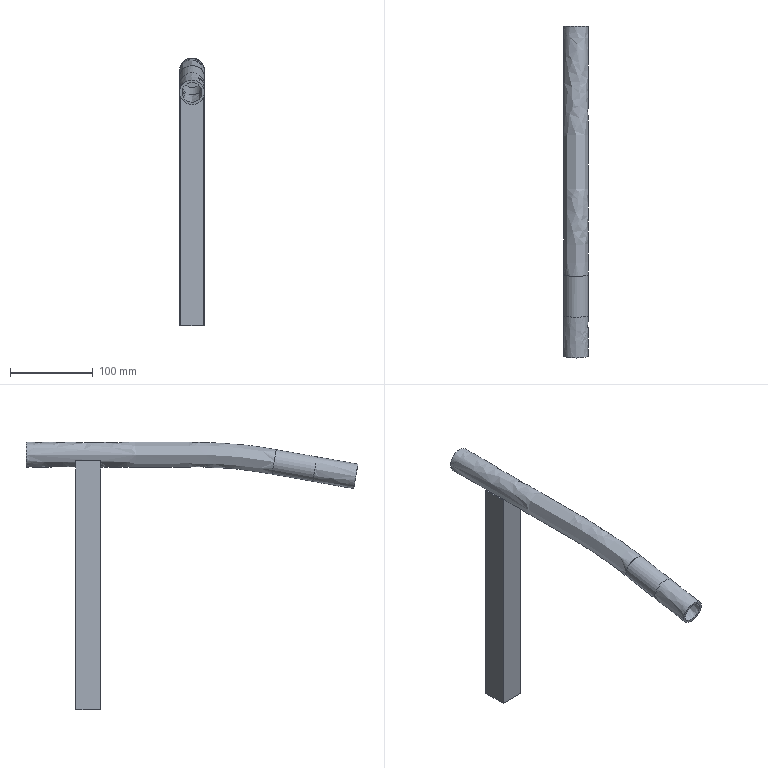Part | NX | features solid 2 | 1 solid | 22 faces | box 30 x 400.326 x 322.586 mm | volume 154131 mm3 | plane 15 | spline 4 | cylinder 3 | commonest cylinder face diameters 30 x2 24 x1
STEP:
#1=CARTESIAN_POINT('',(-652.509,-944.,-115.));
#2=VERTEX_POINT('',#1);
#3=CARTESIAN_POINT('',(-678.491,-944.,-115.));
#4=VERTEX_POINT('',#3);
#5=CARTESIAN_POINT('',(-652.509,-944.,-115.));
#6=CARTESIAN_POINT('',(-653.831,-944.,-117.288));
#7=CARTESIAN_POINT('',(-657.637,-944.,-121.084));
#8=CARTESIAN_POINT('',(-665.504,-944.,-123.205));
#9=CARTESIAN_POINT('',(-673.339,-944.,-121.096));
#10=CARTESIAN_POINT('',(-677.169,-944.,-117.288));
#11=CARTESIAN_POINT('',(-678.491,-944.,-115.));
#12=B_SPLINE_CURVE_WITH_KNOTS('',3,(#5,#6,#7,#8,#9,#10,#11),.UNSPECIFIED.,.F.,.F.,(4,1,1,1,4),(0.,0.007815,0.01563,0.02344,0.03126),.UNSPECIFIED.);
#13=EDGE_CURVE('',#2,#4,#12,.T.);
#14=ORIENTED_EDGE('',*,*,#13,.T.);
#15=CARTESIAN_POINT('',(-680.5,-944.,-115.));
#16=VERTEX_POINT('',#15);
#17=CARTESIAN_POINT('',(-680.5,-944.,-115.));
#18=DIRECTION('',(-1.,0.,0.));
#19=VECTOR('',#18,1000.);
#20=LINE('',#17,#19);
#21=EDGE_CURVE('',#16,#4,#20,.F.);
#22=ORIENTED_EDGE('',*,*,#21,.F.);
#23=CARTESIAN_POINT('',(-680.5,-944.,-415.));
#24=VERTEX_POINT('',#23);
#25=CARTESIAN_POINT('',(-680.5,-944.,-400.));
#26=DIRECTION('',(0.,0.,1.));
#27=VECTOR('',#26,1000.);
#28=LINE('',#25,#27);
#29=EDGE_CURVE('',#24,#16,#28,.T.);
#30=ORIENTED_EDGE('',*,*,#29,.F.);
#31=CARTESIAN_POINT('',(-650.5,-944.,-415.));
#32=VERTEX_POINT('',#31);
#33=CARTESIAN_POINT('',(-683.25,-944.,-415.));
#34=DIRECTION('',(-1.,0.,0.));
#35=VECTOR('',#34,1000.);
#36=LINE('',#33,#35);
#37=EDGE_CURVE('',#24,#32,#36,.F.);
#38=ORIENTED_EDGE('',*,*,#37,.T.);
#39=CARTESIAN_POINT('',(-650.5,-944.,-115.));
#40=VERTEX_POINT('',#39);
#41=CARTESIAN_POINT('',(-650.5,-944.,-400.));
#42=DIRECTION('',(0.,0.,-1.));
#43=VECTOR('',#42,1000.);
#44=LINE('',#41,#43);
#45=EDGE_CURVE('',#32,#40,#44,.F.);
#46=ORIENTED_EDGE('',*,*,#45,.T.);
#47=CARTESIAN_POINT('',(-680.5,-944.,-115.));
#48=DIRECTION('',(-1.,0.,0.));
#49=VECTOR('',#48,1000.);
#50=LINE('',#47,#49);
#51=EDGE_CURVE('',#2,#40,#50,.F.);
#52=ORIENTED_EDGE('',*,*,#51,.F.);
#53=EDGE_LOOP('',(#14,#22,#30,#38,#46,#52));
#54=FACE_BOUND('',#53,.T.);
#55=CARTESIAN_POINT('',(-683.25,-944.,-400.));
#56=DIRECTION('',(0.,1.,0.));
#57=DIRECTION('',(1.,0.,0.));
#58=AXIS2_PLACEMENT_3D('',#55,#56,#57);
#59=PLANE('',#58);
#60=ADVANCED_FACE('',(#54),#59,.F.);
#61=CARTESIAN_POINT('',(-678.49,-942.5,-115.));
#62=VERTEX_POINT('',#61);
#63=CARTESIAN_POINT('',(-652.51,-942.5,-115.));
#64=VERTEX_POINT('',#63);
#65=CARTESIAN_POINT('',(-678.49,-942.5,-115.));
#66=CARTESIAN_POINT('',(-677.169,-942.5,-117.288));
#67=CARTESIAN_POINT('',(-673.363,-942.5,-121.084));
#68=CARTESIAN_POINT('',(-665.496,-942.5,-123.205));
#69=CARTESIAN_POINT('',(-657.661,-942.5,-121.096));
#70=CARTESIAN_POINT('',(-653.831,-942.5,-117.288));
#71=CARTESIAN_POINT('',(-652.51,-942.5,-115.));
#72=B_SPLINE_CURVE_WITH_KNOTS('',3,(#65,#66,#67,#68,#69,#70,#71),.UNSPECIFIED.,.F.,.F.,(4,1,1,1,4),(0.,0.007814,0.01563,0.02344,0.03126),.UNSPECIFIED.);
#73=EDGE_CURVE('',#62,#64,#72,.T.);
#74=ORIENTED_EDGE('',*,*,#73,.T.);
#75=CARTESIAN_POINT('',(-652.,-942.5,-115.));
#76=VERTEX_POINT('',#75);
#77=CARTESIAN_POINT('',(-683.25,-942.5,-115.));
#78=DIRECTION('',(-1.,0.,0.));
#79=VECTOR('',#78,1000.);
#80=LINE('',#77,#79);
#81=EDGE_CURVE('',#76,#64,#80,.T.);
#82=ORIENTED_EDGE('',*,*,#81,.F.);
#83=CARTESIAN_POINT('',(-652.,-942.5,-415.));
#84=VERTEX_POINT('',#83);
#85=CARTESIAN_POINT('',(-652.,-942.5,-50.));
#86=DIRECTION('',(0.,0.,-1.));
#87=VECTOR('',#86,1000.);
#88=LINE('',#85,#87);
#89=EDGE_CURVE('',#76,#84,#88,.T.);
#90=ORIENTED_EDGE('',*,*,#89,.T.);
#91=CARTESIAN_POINT('',(-679.,-942.5,-415.));
#92=VERTEX_POINT('',#91);
#93=CARTESIAN_POINT('',(-683.25,-942.5,-415.));
#94=DIRECTION('',(1.,0.,0.));
#95=VECTOR('',#94,1000.);
#96=LINE('',#93,#95);
#97=EDGE_CURVE('',#84,#92,#96,.F.);
#98=ORIENTED_EDGE('',*,*,#97,.T.);
#99=CARTESIAN_POINT('',(-679.,-942.5,-115.));
#100=VERTEX_POINT('',#99);
#101=CARTESIAN_POINT('',(-679.,-942.5,-50.));
#102=DIRECTION('',(0.,0.,-1.));
#103=VECTOR('',#102,1000.);
#104=LINE('',#101,#103);
#105=EDGE_CURVE('',#100,#92,#104,.T.);
#106=ORIENTED_EDGE('',*,*,#105,.F.);
#107=CARTESIAN_POINT('',(-683.25,-942.5,-115.));
#108=DIRECTION('',(-1.,0.,0.));
#109=VECTOR('',#108,1000.);
#110=LINE('',#107,#109);
#111=EDGE_CURVE('',#62,#100,#110,.T.);
#112=ORIENTED_EDGE('',*,*,#111,.F.);
#113=EDGE_LOOP('',(#74,#82,#90,#98,#106,#112));
#114=FACE_BOUND('',#113,.T.);
#115=CARTESIAN_POINT('',(-683.25,-942.5,-50.));
#116=DIRECTION('',(0.,-1.,0.));
#117=DIRECTION('',(-1.,0.,0.));
#118=AXIS2_PLACEMENT_3D('',#115,#116,#117);
#119=PLANE('',#118);
#120=ADVANCED_FACE('',(#114),#119,.F.);
#121=CARTESIAN_POINT('',(-652.509,-944.,-115.));
#122=CARTESIAN_POINT('',(-652.51,-943.5,-115.));
#123=CARTESIAN_POINT('',(-652.51,-943.,-115.));
#124=CARTESIAN_POINT('',(-652.51,-942.5,-115.));
#125=B_SPLINE_CURVE_WITH_KNOTS('',3,(#121,#122,#123,#124),.UNSPECIFIED.,.F.,.F.,(4,4),(0.,0.0015),.UNSPECIFIED.);
#126=EDGE_CURVE('',#64,#2,#125,.F.);
#127=ORIENTED_EDGE('',*,*,#126,.T.);
#128=ORIENTED_EDGE('',*,*,#51,.T.);
#129=CARTESIAN_POINT('',(-650.5,-914.,-115.));
#130=VERTEX_POINT('',#129);
#131=CARTESIAN_POINT('',(-650.5,-914.,-115.));
#132=DIRECTION('',(0.,-1.,0.));
#133=VECTOR('',#132,1000.);
#134=LINE('',#131,#133);
#135=EDGE_CURVE('',#40,#130,#134,.F.);
#136=ORIENTED_EDGE('',*,*,#135,.T.);
#137=CARTESIAN_POINT('',(-652.51,-914.,-115.));
#138=VERTEX_POINT('',#137);
#139=CARTESIAN_POINT('',(-680.5,-914.,-115.));
#140=DIRECTION('',(-1.,0.,0.));
#141=VECTOR('',#140,1000.);
#142=LINE('',#139,#141);
#143=EDGE_CURVE('',#138,#130,#142,.F.);
#144=ORIENTED_EDGE('',*,*,#143,.F.);
#145=CARTESIAN_POINT('',(-652.51,-915.5,-115.));
#146=VERTEX_POINT('',#145);
#147=CARTESIAN_POINT('',(-652.51,-544.,-115.));
#148=DIRECTION('',(0.,-1.,0.));
#149=VECTOR('',#148,1000.);
#150=LINE('',#147,#149);
#151=EDGE_CURVE('',#138,#146,#150,.T.);
#152=ORIENTED_EDGE('',*,*,#151,.T.);
#153=CARTESIAN_POINT('',(-652.,-915.5,-115.));
#154=VERTEX_POINT('',#153);
#155=CARTESIAN_POINT('',(-683.25,-915.5,-115.));
#156=DIRECTION('',(-1.,0.,0.));
#157=VECTOR('',#156,1000.);
#158=LINE('',#155,#157);
#159=EDGE_CURVE('',#154,#146,#158,.T.);
#160=ORIENTED_EDGE('',*,*,#159,.F.);
#161=CARTESIAN_POINT('',(-652.,-914.,-115.));
#162=DIRECTION('',(0.,1.,0.));
#163=VECTOR('',#162,1000.);
#164=LINE('',#161,#163);
#165=EDGE_CURVE('',#76,#154,#164,.T.);
#166=ORIENTED_EDGE('',*,*,#165,.F.);
#167=ORIENTED_EDGE('',*,*,#81,.T.);
#168=EDGE_LOOP('',(#127,#128,#136,#144,#152,#160,#166,#167));
#169=FACE_BOUND('',#168,.T.);
#170=CARTESIAN_POINT('',(-680.5,-914.,-115.));
#171=DIRECTION('',(0.,0.,-1.));
#172=DIRECTION('',(0.,1.,0.));
#173=AXIS2_PLACEMENT_3D('',#170,#171,#172);
#174=PLANE('',#173);
#175=ADVANCED_FACE('',(#169),#174,.F.);
#176=CARTESIAN_POINT('',(-678.491,-944.,-115.));
#177=CARTESIAN_POINT('',(-678.49,-943.5,-115.));
#178=CARTESIAN_POINT('',(-678.49,-943.,-115.));
#179=CARTESIAN_POINT('',(-678.49,-942.5,-115.));
#180=B_SPLINE_CURVE_WITH_KNOTS('',3,(#176,#177,#178,#179),.UNSPECIFIED.,.F.,.F.,(4,4),(0.,0.0015),.UNSPECIFIED.);
#181=EDGE_CURVE('',#4,#62,#180,.T.);
#182=ORIENTED_EDGE('',*,*,#181,.T.);
#183=ORIENTED_EDGE('',*,*,#111,.T.);
#184=CARTESIAN_POINT('',(-679.,-915.5,-115.));
#185=VERTEX_POINT('',#184);
#186=CARTESIAN_POINT('',(-679.,-914.,-115.));
#187=DIRECTION('',(0.,1.,0.));
#188=VECTOR('',#187,1000.);
#189=LINE('',#186,#188);
#190=EDGE_CURVE('',#100,#185,#189,.T.);
#191=ORIENTED_EDGE('',*,*,#190,.T.);
#192=CARTESIAN_POINT('',(-678.49,-915.5,-115.));
#193=VERTEX_POINT('',#192);
#194=CARTESIAN_POINT('',(-683.25,-915.5,-115.));
#195=DIRECTION('',(-1.,0.,0.));
#196=VECTOR('',#195,1000.);
#197=LINE('',#194,#196);
#198=EDGE_CURVE('',#193,#185,#197,.T.);
#199=ORIENTED_EDGE('',*,*,#198,.F.);
#200=CARTESIAN_POINT('',(-678.49,-914.,-115.));
#201=VERTEX_POINT('',#200);
#202=CARTESIAN_POINT('',(-678.49,-544.,-115.));
#203=DIRECTION('',(0.,-1.,0.));
#204=VECTOR('',#203,1000.);
#205=LINE('',#202,#204);
#206=EDGE_CURVE('',#193,#201,#205,.F.);
#207=ORIENTED_EDGE('',*,*,#206,.T.);
#208=CARTESIAN_POINT('',(-680.5,-914.,-115.));
#209=VERTEX_POINT('',#208);
#210=CARTESIAN_POINT('',(-680.5,-914.,-115.));
#211=DIRECTION('',(-1.,0.,0.));
#212=VECTOR('',#211,1000.);
#213=LINE('',#210,#212);
#214=EDGE_CURVE('',#209,#201,#213,.F.);
#215=ORIENTED_EDGE('',*,*,#214,.F.);
#216=CARTESIAN_POINT('',(-680.5,-914.,-115.));
#217=DIRECTION('',(0.,1.,0.));
#218=VECTOR('',#217,1000.);
#219=LINE('',#216,#218);
#220=EDGE_CURVE('',#209,#16,#219,.F.);
#221=ORIENTED_EDGE('',*,*,#220,.T.);
#222=ORIENTED_EDGE('',*,*,#21,.T.);
#223=EDGE_LOOP('',(#182,#183,#191,#199,#207,#215,#221,#222));
#224=FACE_BOUND('',#223,.T.);
#225=CARTESIAN_POINT('',(-680.5,-914.,-115.));
#226=DIRECTION('',(0.,0.,-1.));
#227=DIRECTION('',(0.,1.,0.));
#228=AXIS2_PLACEMENT_3D('',#225,#226,#227);
#229=PLANE('',#228);
#230=ADVANCED_FACE('',(#224),#229,.F.);
#231=CARTESIAN_POINT('',(-680.5,-914.,-415.));
#232=VERTEX_POINT('',#231);
#233=CARTESIAN_POINT('',(-680.5,-914.,-415.));
#234=DIRECTION('',(0.,1.,0.));
#235=VECTOR('',#234,1000.);
#236=LINE('',#233,#235);
#237=EDGE_CURVE('',#232,#24,#236,.F.);
#238=ORIENTED_EDGE('',*,*,#237,.F.);
#239=CARTESIAN_POINT('',(-650.5,-914.,-415.));
#240=VERTEX_POINT('',#239);
#241=CARTESIAN_POINT('',(-683.25,-914.,-415.));
#242=DIRECTION('',(-1.,0.,0.));
#243=VECTOR('',#242,1000.);
#244=LINE('',#241,#243);
#245=EDGE_CURVE('',#232,#240,#244,.F.);
#246=ORIENTED_EDGE('',*,*,#245,.T.);
#247=CARTESIAN_POINT('',(-650.5,-914.,-415.));
#248=DIRECTION('',(0.,-1.,0.));
#249=VECTOR('',#248,1000.);
#250=LINE('',#247,#249);
#251=EDGE_CURVE('',#240,#32,#250,.T.);
#252=ORIENTED_EDGE('',*,*,#251,.T.);
#253=ORIENTED_EDGE('',*,*,#37,.F.);
#254=EDGE_LOOP('',(#238,#246,#252,#253));
#255=FACE_BOUND('',#254,.T.);
#256=CARTESIAN_POINT('',(-652.,-915.5,-415.));
#257=VERTEX_POINT('',#256);
#258=CARTESIAN_POINT('',(-652.,-914.,-415.));
#259=DIRECTION('',(0.,-1.,0.));
#260=VECTOR('',#259,1000.);
#261=LINE('',#258,#260);
#262=EDGE_CURVE('',#84,#257,#261,.F.);
#263=ORIENTED_EDGE('',*,*,#262,.T.);
#264=CARTESIAN_POINT('',(-679.,-915.5,-415.));
#265=VERTEX_POINT('',#264);
#266=CARTESIAN_POINT('',(-683.25,-915.5,-415.));
#267=DIRECTION('',(1.,0.,0.));
#268=VECTOR('',#267,1000.);
#269=LINE('',#266,#268);
#270=EDGE_CURVE('',#257,#265,#269,.F.);
#271=ORIENTED_EDGE('',*,*,#270,.T.);
#272=CARTESIAN_POINT('',(-679.,-914.,-415.));
#273=DIRECTION('',(0.,-1.,0.));
#274=VECTOR('',#273,1000.);
#275=LINE('',#272,#274);
#276=EDGE_CURVE('',#92,#265,#275,.F.);
#277=ORIENTED_EDGE('',*,*,#276,.F.);
#278=ORIENTED_EDGE('',*,*,#97,.F.);
#279=EDGE_LOOP('',(#263,#271,#277,#278));
#280=FACE_BOUND('',#279,.T.);
#281=CARTESIAN_POINT('',(-683.25,-914.,-415.));
#282=DIRECTION('',(0.,0.,-1.));
#283=DIRECTION('',(1.,0.,0.));
#284=AXIS2_PLACEMENT_3D('',#281,#282,#283);
#285=PLANE('',#284);
#286=ADVANCED_FACE('',(#255,#280),#285,.T.);
#287=ORIENTED_EDGE('',*,*,#45,.F.);
#288=ORIENTED_EDGE('',*,*,#251,.F.);
#289=CARTESIAN_POINT('',(-650.5,-914.,-400.));
#290=DIRECTION('',(0.,0.,-1.));
#291=VECTOR('',#290,1000.);
#292=LINE('',#289,#291);
#293=EDGE_CURVE('',#240,#130,#292,.F.);
#294=ORIENTED_EDGE('',*,*,#293,.T.);
#295=ORIENTED_EDGE('',*,*,#135,.F.);
#296=EDGE_LOOP('',(#287,#288,#294,#295));
#297=FACE_BOUND('',#296,.T.);
#298=CARTESIAN_POINT('',(-650.5,-914.,-400.));
#299=DIRECTION('',(1.,0.,0.));
#300=DIRECTION('',(0.,0.,1.));
#301=AXIS2_PLACEMENT_3D('',#298,#299,#300);
#302=PLANE('',#301);
#303=ADVANCED_FACE('',(#297),#302,.T.);
#304=CARTESIAN_POINT('',(-680.5,-914.,-400.));
#305=DIRECTION('',(0.,0.,1.));
#306=VECTOR('',#305,1000.);
#307=LINE('',#304,#306);
#308=EDGE_CURVE('',#232,#209,#307,.T.);
#309=ORIENTED_EDGE('',*,*,#308,.F.);
#310=ORIENTED_EDGE('',*,*,#237,.T.);
#311=ORIENTED_EDGE('',*,*,#29,.T.);
#312=ORIENTED_EDGE('',*,*,#220,.F.);
#313=EDGE_LOOP('',(#309,#310,#311,#312));
#314=FACE_BOUND('',#313,.T.);
#315=CARTESIAN_POINT('',(-680.5,-914.,-400.));
#316=DIRECTION('',(1.,0.,0.));
#317=DIRECTION('',(0.,0.,1.));
#318=AXIS2_PLACEMENT_3D('',#315,#316,#317);
#319=PLANE('',#318);
#320=ADVANCED_FACE('',(#314),#319,.F.);
#321=ORIENTED_EDGE('',*,*,#214,.T.);
#322=CARTESIAN_POINT('',(-665.5,-914.,-107.5));
#323=DIRECTION('',(0.,-1.,0.));
#324=DIRECTION('',(1.,0.,0.));
#325=AXIS2_PLACEMENT_3D('',#322,#323,#324);
#326=CIRCLE('',#325,15.);
#327=EDGE_CURVE('',#201,#138,#326,.T.);
#328=ORIENTED_EDGE('',*,*,#327,.T.);
#329=ORIENTED_EDGE('',*,*,#143,.T.);
#330=ORIENTED_EDGE('',*,*,#293,.F.);
#331=ORIENTED_EDGE('',*,*,#245,.F.);
#332=ORIENTED_EDGE('',*,*,#308,.T.);
#333=EDGE_LOOP('',(#321,#328,#329,#330,#331,#332));
#334=FACE_BOUND('',#333,.T.);
#335=CARTESIAN_POINT('',(-683.25,-914.,-400.));
#336=DIRECTION('',(0.,1.,0.));
#337=DIRECTION('',(1.,0.,0.));
#338=AXIS2_PLACEMENT_3D('',#335,#336,#337);
#339=PLANE('',#338);
#340=ADVANCED_FACE('',(#334),#339,.T.);
#341=ORIENTED_EDGE('',*,*,#165,.T.);
#342=CARTESIAN_POINT('',(-652.,-915.5,-50.));
#343=DIRECTION('',(0.,0.,-1.));
#344=VECTOR('',#343,1000.);
#345=LINE('',#342,#344);
#346=EDGE_CURVE('',#154,#257,#345,.T.);
#347=ORIENTED_EDGE('',*,*,#346,.T.);
#348=ORIENTED_EDGE('',*,*,#262,.F.);
#349=ORIENTED_EDGE('',*,*,#89,.F.);
#350=EDGE_LOOP('',(#341,#347,#348,#349));
#351=FACE_BOUND('',#350,.T.);
#352=CARTESIAN_POINT('',(-652.,-914.,-50.));
#353=DIRECTION('',(-1.,0.,0.));
#354=DIRECTION('',(0.,1.,0.));
#355=AXIS2_PLACEMENT_3D('',#352,#353,#354);
#356=PLANE('',#355);
#357=ADVANCED_FACE('',(#351),#356,.T.);
#358=ORIENTED_EDGE('',*,*,#105,.T.);
#359=ORIENTED_EDGE('',*,*,#276,.T.);
#360=CARTESIAN_POINT('',(-679.,-915.5,-50.));
#361=DIRECTION('',(0.,0.,-1.));
#362=VECTOR('',#361,1000.);
#363=LINE('',#360,#362);
#364=EDGE_CURVE('',#185,#265,#363,.T.);
#365=ORIENTED_EDGE('',*,*,#364,.F.);
#366=ORIENTED_EDGE('',*,*,#190,.F.);
#367=EDGE_LOOP('',(#358,#359,#365,#366));
#368=FACE_BOUND('',#367,.T.);
#369=CARTESIAN_POINT('',(-679.,-914.,-50.));
#370=DIRECTION('',(-1.,0.,0.));
#371=DIRECTION('',(0.,1.,0.));
#372=AXIS2_PLACEMENT_3D('',#369,#370,#371);
#373=PLANE('',#372);
#374=ADVANCED_FACE('',(#368),#373,.F.);
#375=ORIENTED_EDGE('',*,*,#159,.T.);
#376=CARTESIAN_POINT('',(-665.5,-915.5,-107.5));
#377=DIRECTION('',(0.,1.,0.));
#378=DIRECTION('',(-1.,0.,0.));
#379=AXIS2_PLACEMENT_3D('',#376,#377,#378);
#380=CIRCLE('',#379,15.);
#381=EDGE_CURVE('',#146,#193,#380,.T.);
#382=ORIENTED_EDGE('',*,*,#381,.T.);
#383=ORIENTED_EDGE('',*,*,#198,.T.);
#384=ORIENTED_EDGE('',*,*,#364,.T.);
#385=ORIENTED_EDGE('',*,*,#270,.F.);
#386=ORIENTED_EDGE('',*,*,#346,.F.);
#387=EDGE_LOOP('',(#375,#382,#383,#384,#385,#386));
#388=FACE_BOUND('',#387,.T.);
#389=CARTESIAN_POINT('',(-683.25,-915.5,-50.));
#390=DIRECTION('',(0.,-1.,0.));
#391=DIRECTION('',(-1.,0.,0.));
#392=AXIS2_PLACEMENT_3D('',#389,#390,#391);
#393=PLANE('',#392);
#394=ADVANCED_FACE('',(#388),#393,.T.);
#395=ORIENTED_EDGE('',*,*,#381,.F.);
#396=ORIENTED_EDGE('',*,*,#151,.F.);
#397=ORIENTED_EDGE('',*,*,#327,.F.);
#398=ORIENTED_EDGE('',*,*,#206,.F.);
#399=EDGE_LOOP('',(#395,#396,#397,#398));
#400=FACE_BOUND('',#399,.T.);
#401=CARTESIAN_POINT('',(-665.5,-544.,-107.5));
#402=DIRECTION('',(0.,-1.,0.));
#403=DIRECTION('',(-1.,0.,0.));
#404=AXIS2_PLACEMENT_3D('',#401,#402,#403);
#405=CYLINDRICAL_SURFACE('',#404,15.);
#406=ADVANCED_FACE('',(#400),#405,.F.);
#407=CARTESIAN_POINT('',(-650.583,-854.,-109.075));
#408=VERTEX_POINT('',#407);
#409=CARTESIAN_POINT('',(-651.992,-854.,-114.869));
#410=CARTESIAN_POINT('',(-649.578,-854.,-107.193));
#411=CARTESIAN_POINT('',(-652.578,-854.,-97.049));
#412=CARTESIAN_POINT('',(-663.744,-854.,-90.971));
#413=CARTESIAN_POINT('',(-675.949,-854.,-94.569));
#414=CARTESIAN_POINT('',(-682.029,-854.,-105.753));
#415=CARTESIAN_POINT('',(-678.434,-854.,-117.937));
#416=CARTESIAN_POINT('',(-667.26,-854.,-124.035));
#417=CARTESIAN_POINT('',(-657.101,-854.,-121.018));
#418=CARTESIAN_POINT('',(-651.992,-854.,-114.869));
#419=CARTESIAN_POINT('',(-649.578,-854.,-107.193));
#420=CARTESIAN_POINT('',(-652.578,-854.,-97.049));
#421=B_SPLINE_CURVE_WITH_KNOTS('',3,(#409,#410,#411,#412,#413,#414,#415,#416,#417,#418,#419,#420),.UNSPECIFIED.,.T.,.F.,(1,1,1,1,1,1,1,1,1,1,1,1,1,1,1,1),(-0.02345,-0.01172,-0.005861,0.,0.01172,0.02345,0.03517,0.04689,0.05861,0.07034,0.08206,0.08792,0.09378,0.1055,0.1172,0.129),.UNSPECIFIED.);
#422=EDGE_CURVE('',#408,#408,#421,.T.);
#423=ORIENTED_EDGE('',*,*,#422,.T.);
#424=EDGE_LOOP('',(#423));
#425=FACE_BOUND('',#424,.T.);
#426=CARTESIAN_POINT('',(-680.5,-1153.241,-116.177));
#427=VERTEX_POINT('',#426);
#428=CARTESIAN_POINT('',(-650.5,-1153.241,-116.177));
#429=VERTEX_POINT('',#428);
#430=CARTESIAN_POINT('',(-680.5,-1153.241,-116.177));
#431=CARTESIAN_POINT('',(-680.499,-1152.897,-118.128));
#432=CARTESIAN_POINT('',(-679.714,-1152.22,-121.97));
#433=CARTESIAN_POINT('',(-675.273,-1151.06,-128.546));
#434=CARTESIAN_POINT('',(-665.515,-1150.356,-132.54));
#435=CARTESIAN_POINT('',(-653.749,-1151.2,-127.754));
#436=CARTESIAN_POINT('',(-650.501,-1152.562,-120.032));
#437=CARTESIAN_POINT('',(-650.5,-1153.241,-116.177));
#438=B_SPLINE_CURVE_WITH_KNOTS('',3,(#430,#431,#432,#433,#434,#435,#436,#437),.UNSPECIFIED.,.F.,.F.,(4,1,1,1,1,4),(0.000005601,0.005866,0.01173,0.02345,0.03517,0.04689),.UNSPECIFIED.);
#439=EDGE_CURVE('',#427,#429,#438,.T.);
#440=ORIENTED_EDGE('',*,*,#439,.F.);
#441=CARTESIAN_POINT('',(-650.5,-1153.241,-116.177));
#442=CARTESIAN_POINT('',(-650.499,-1153.921,-112.32));
#443=CARTESIAN_POINT('',(-653.734,-1155.281,-104.61));
#444=CARTESIAN_POINT('',(-665.485,-1156.13,-99.795));
#445=CARTESIAN_POINT('',(-677.248,-1155.282,-104.605));
#446=CARTESIAN_POINT('',(-680.502,-1153.93,-112.273));
#447=CARTESIAN_POINT('',(-680.5,-1153.241,-116.177));
#448=B_SPLINE_CURVE_WITH_KNOTS('',3,(#441,#442,#443,#444,#445,#446,#447),.UNSPECIFIED.,.F.,.F.,(4,1,1,1,4),(0.04689,0.05862,0.07034,0.08206,0.09379),.UNSPECIFIED.);
#449=EDGE_CURVE('',#429,#427,#448,.T.);
#450=ORIENTED_EDGE('',*,*,#449,.F.);
#451=EDGE_LOOP('',(#440,#450));
#452=FACE_BOUND('',#451,.T.);
#453=ORIENTED_EDGE('',*,*,#73,.F.);
#454=ORIENTED_EDGE('',*,*,#181,.F.);
#455=ORIENTED_EDGE('',*,*,#13,.F.);
#456=ORIENTED_EDGE('',*,*,#126,.F.);
#457=EDGE_LOOP('',(#453,#454,#455,#456));
#458=FACE_BOUND('',#457,.T.);
#459=CARTESIAN_POINT('',(-680.5,-854.,-102.197));
#460=CARTESIAN_POINT('',(-680.5,-883.148,-102.197));
#461=CARTESIAN_POINT('',(-680.5,-926.87,-102.193));
#462=CARTESIAN_POINT('',(-680.5,-985.165,-102.202));
#463=CARTESIAN_POINT('',(-680.5,-1021.586,-102.198));
#464=CARTESIAN_POINT('',(-680.5,-1050.761,-102.064));
#465=CARTESIAN_POINT('',(-680.5,-1080.089,-102.334));
#466=CARTESIAN_POINT('',(-680.5,-1109.539,-104.218));
#467=CARTESIAN_POINT('',(-680.5,-1137.275,-107.994));
#468=CARTESIAN_POINT('',(-680.5,-1150.26,-110.257));
#469=CARTESIAN_POINT('',(-680.5,-1156.026,-111.278));
#470=CARTESIAN_POINT('',(-680.5,-854.,-112.803));
#471=CARTESIAN_POINT('',(-680.5,-883.148,-112.803));
#472=CARTESIAN_POINT('',(-680.5,-926.869,-112.8));
#473=CARTESIAN_POINT('',(-680.5,-985.165,-112.809));
#474=CARTESIAN_POINT('',(-680.5,-1021.611,-112.805));
#475=CARTESIAN_POINT('',(-680.5,-1050.737,-112.671));
#476=CARTESIAN_POINT('',(-680.5,-1079.701,-112.937));
#477=CARTESIAN_POINT('',(-680.5,-1108.483,-114.779));
#478=CARTESIAN_POINT('',(-680.5,-1135.656,-118.478));
#479=CARTESIAN_POINT('',(-680.5,-1148.533,-120.723));
#480=CARTESIAN_POINT('',(-680.5,-1154.267,-121.738));
#481=CARTESIAN_POINT('',(-677.848,-854.,-119.848));
#482=CARTESIAN_POINT('',(-677.848,-883.148,-119.848));
#483=CARTESIAN_POINT('',(-677.848,-926.869,-119.845));
#484=CARTESIAN_POINT('',(-677.848,-985.165,-119.854));
#485=CARTESIAN_POINT('',(-677.848,-1021.628,-119.85));
#486=CARTESIAN_POINT('',(-677.848,-1050.721,-119.716));
#487=CARTESIAN_POINT('',(-677.848,-1079.443,-119.98));
#488=CARTESIAN_POINT('',(-677.848,-1107.782,-121.794));
#489=CARTESIAN_POINT('',(-677.848,-1134.581,-125.442));
#490=CARTESIAN_POINT('',(-677.848,-1147.387,-127.674));
#491=CARTESIAN_POINT('',(-677.848,-1153.098,-128.686));
#492=CARTESIAN_POINT('',(-670.803,-854.,-122.5));
#493=CARTESIAN_POINT('',(-670.803,-883.148,-122.5));
#494=CARTESIAN_POINT('',(-670.803,-926.869,-122.497));
#495=CARTESIAN_POINT('',(-670.803,-985.165,-122.506));
#496=CARTESIAN_POINT('',(-670.803,-1021.634,-122.502));
#497=CARTESIAN_POINT('',(-670.803,-1050.715,-122.368));
#498=CARTESIAN_POINT('',(-670.803,-1079.346,-122.631));
#499=CARTESIAN_POINT('',(-670.803,-1107.519,-124.434));
#500=CARTESIAN_POINT('',(-670.803,-1134.177,-128.063));
#501=CARTESIAN_POINT('',(-670.803,-1146.955,-130.291));
#502=CARTESIAN_POINT('',(-670.803,-1152.659,-131.301));
#503=CARTESIAN_POINT('',(-660.197,-854.,-122.5));
#504=CARTESIAN_POINT('',(-660.197,-883.148,-122.5));
#505=CARTESIAN_POINT('',(-660.197,-926.869,-122.497));
#506=CARTESIAN_POINT('',(-660.197,-985.165,-122.506));
#507=CARTESIAN_POINT('',(-660.197,-1021.634,-122.502));
#508=CARTESIAN_POINT('',(-660.197,-1050.715,-122.368));
#509=CARTESIAN_POINT('',(-660.197,-1079.346,-122.631));
#510=CARTESIAN_POINT('',(-660.197,-1107.519,-124.434));
#511=CARTESIAN_POINT('',(-660.197,-1134.177,-128.063));
#512=CARTESIAN_POINT('',(-660.197,-1146.955,-130.291));
#513=CARTESIAN_POINT('',(-660.197,-1152.659,-131.301));
#514=CARTESIAN_POINT('',(-653.152,-854.,-119.848));
#515=CARTESIAN_POINT('',(-653.152,-883.148,-119.848));
#516=CARTESIAN_POINT('',(-653.152,-926.869,-119.845));
#517=CARTESIAN_POINT('',(-653.152,-985.165,-119.854));
#518=CARTESIAN_POINT('',(-653.152,-1021.628,-119.85));
#519=CARTESIAN_POINT('',(-653.152,-1050.721,-119.716));
#520=CARTESIAN_POINT('',(-653.152,-1079.443,-119.98));
#521=CARTESIAN_POINT('',(-653.152,-1107.782,-121.794));
#522=CARTESIAN_POINT('',(-653.152,-1134.581,-125.442));
#523=CARTESIAN_POINT('',(-653.152,-1147.387,-127.674));
#524=CARTESIAN_POINT('',(-653.152,-1153.098,-128.686));
#525=CARTESIAN_POINT('',(-650.5,-854.,-112.803));
#526=CARTESIAN_POINT('',(-650.5,-883.148,-112.803));
#527=CARTESIAN_POINT('',(-650.5,-926.869,-112.8));
#528=CARTESIAN_POINT('',(-650.5,-985.165,-112.809));
#529=CARTESIAN_POINT('',(-650.5,-1021.611,-112.805));
#530=CARTESIAN_POINT('',(-650.5,-1050.737,-112.671));
#531=CARTESIAN_POINT('',(-650.5,-1079.701,-112.937));
#532=CARTESIAN_POINT('',(-650.5,-1108.483,-114.779));
#533=CARTESIAN_POINT('',(-650.5,-1135.656,-118.478));
#534=CARTESIAN_POINT('',(-650.5,-1148.533,-120.723));
#535=CARTESIAN_POINT('',(-650.5,-1154.267,-121.738));
#536=CARTESIAN_POINT('',(-650.5,-854.,-102.197));
#537=CARTESIAN_POINT('',(-650.5,-883.148,-102.197));
#538=CARTESIAN_POINT('',(-650.5,-926.87,-102.193));
#539=CARTESIAN_POINT('',(-650.5,-985.165,-102.202));
#540=CARTESIAN_POINT('',(-650.5,-1021.586,-102.198));
#541=CARTESIAN_POINT('',(-650.5,-1050.761,-102.064));
#542=CARTESIAN_POINT('',(-650.5,-1080.089,-102.334));
#543=CARTESIAN_POINT('',(-650.5,-1109.539,-104.218));
#544=CARTESIAN_POINT('',(-650.5,-1137.275,-107.994));
#545=CARTESIAN_POINT('',(-650.5,-1150.26,-110.257));
#546=CARTESIAN_POINT('',(-650.5,-1156.026,-111.278));
#547=CARTESIAN_POINT('',(-653.152,-854.,-95.152));
#548=CARTESIAN_POINT('',(-653.152,-883.147,-95.152));
#549=CARTESIAN_POINT('',(-653.152,-926.87,-95.148));
#550=CARTESIAN_POINT('',(-653.152,-985.165,-95.157));
#551=CARTESIAN_POINT('',(-653.152,-1021.57,-95.153));
#552=CARTESIAN_POINT('',(-653.152,-1050.778,-95.019));
#553=CARTESIAN_POINT('',(-653.152,-1080.346,-95.291));
#554=CARTESIAN_POINT('',(-653.152,-1110.24,-97.204));
#555=CARTESIAN_POINT('',(-653.152,-1138.35,-101.03));
#556=CARTESIAN_POINT('',(-653.152,-1151.407,-103.305));
#557=CARTESIAN_POINT('',(-653.152,-1157.194,-104.33));
#558=CARTESIAN_POINT('',(-660.197,-854.,-92.5));
#559=CARTESIAN_POINT('',(-660.197,-883.147,-92.5));
#560=CARTESIAN_POINT('',(-660.197,-926.87,-92.497));
#561=CARTESIAN_POINT('',(-660.197,-985.165,-92.506));
#562=CARTESIAN_POINT('',(-660.197,-1021.564,-92.502));
#563=CARTESIAN_POINT('',(-660.197,-1050.784,-92.368));
#564=CARTESIAN_POINT('',(-660.197,-1080.443,-92.64));
#565=CARTESIAN_POINT('',(-660.197,-1110.503,-94.564));
#566=CARTESIAN_POINT('',(-660.197,-1138.755,-98.409));
#567=CARTESIAN_POINT('',(-660.197,-1151.839,-100.689));
#568=CARTESIAN_POINT('',(-660.197,-1157.634,-101.715));
#569=CARTESIAN_POINT('',(-670.803,-854.,-92.5));
#570=CARTESIAN_POINT('',(-670.803,-883.147,-92.5));
#571=CARTESIAN_POINT('',(-670.803,-926.87,-92.497));
#572=CARTESIAN_POINT('',(-670.803,-985.165,-92.506));
#573=CARTESIAN_POINT('',(-670.803,-1021.564,-92.502));
#574=CARTESIAN_POINT('',(-670.803,-1050.784,-92.368));
#575=CARTESIAN_POINT('',(-670.803,-1080.443,-92.64));
#576=CARTESIAN_POINT('',(-670.803,-1110.503,-94.564));
#577=CARTESIAN_POINT('',(-670.803,-1138.755,-98.409));
#578=CARTESIAN_POINT('',(-670.803,-1151.839,-100.689));
#579=CARTESIAN_POINT('',(-670.803,-1157.634,-101.715));
#580=CARTESIAN_POINT('',(-677.848,-854.,-95.152));
#581=CARTESIAN_POINT('',(-677.848,-883.147,-95.152));
#582=CARTESIAN_POINT('',(-677.848,-926.87,-95.148));
#583=CARTESIAN_POINT('',(-677.848,-985.165,-95.157));
#584=CARTESIAN_POINT('',(-677.848,-1021.57,-95.153));
#585=CARTESIAN_POINT('',(-677.848,-1050.778,-95.019));
#586=CARTESIAN_POINT('',(-677.848,-1080.346,-95.291));
#587=CARTESIAN_POINT('',(-677.848,-1110.24,-97.204));
#588=CARTESIAN_POINT('',(-677.848,-1138.35,-101.03));
#589=CARTESIAN_POINT('',(-677.848,-1151.407,-103.305));
#590=CARTESIAN_POINT('',(-677.848,-1157.194,-104.33));
#591=CARTESIAN_POINT('',(-680.5,-854.,-102.197));
#592=CARTESIAN_POINT('',(-680.5,-883.148,-102.197));
#593=CARTESIAN_POINT('',(-680.5,-926.87,-102.193));
#594=CARTESIAN_POINT('',(-680.5,-985.165,-102.202));
#595=CARTESIAN_POINT('',(-680.5,-1021.586,-102.198));
#596=CARTESIAN_POINT('',(-680.5,-1050.761,-102.064));
#597=CARTESIAN_POINT('',(-680.5,-1080.089,-102.334));
#598=CARTESIAN_POINT('',(-680.5,-1109.539,-104.218));
#599=CARTESIAN_POINT('',(-680.5,-1137.275,-107.994));
#600=CARTESIAN_POINT('',(-680.5,-1150.26,-110.257));
#601=CARTESIAN_POINT('',(-680.5,-1156.026,-111.278));
#602=CARTESIAN_POINT('',(-680.5,-854.,-112.803));
#603=CARTESIAN_POINT('',(-680.5,-883.148,-112.803));
#604=CARTESIAN_POINT('',(-680.5,-926.869,-112.8));
#605=CARTESIAN_POINT('',(-680.5,-985.165,-112.809));
#606=CARTESIAN_POINT('',(-680.5,-1021.611,-112.805));
#607=CARTESIAN_POINT('',(-680.5,-1050.737,-112.671));
#608=CARTESIAN_POINT('',(-680.5,-1079.701,-112.937));
#609=CARTESIAN_POINT('',(-680.5,-1108.483,-114.779));
#610=CARTESIAN_POINT('',(-680.5,-1135.656,-118.478));
#611=CARTESIAN_POINT('',(-680.5,-1148.533,-120.723));
#612=CARTESIAN_POINT('',(-680.5,-1154.267,-121.738));
#613=(BOUNDED_SURFACE()B_SPLINE_SURFACE(4,3,((#459,#460,#461,#462,#463,#464,#465,#466,#467,#468,#469),(#470,#471,#472,#473,#474,#475,#476,#477,#478,#479,#480),(#481,#482,#483,#484,#485,#486,#487,#488,#489,#490,#491),(#492,#493,#494,#495,#496,#497,#498,#499,#500,#501,#502),(#503,#504,#505,#506,#507,#508,#509,#510,#511,#512,#513),(#514,#515,#516,#517,#518,#519,#520,#521,#522,#523,#524),(#525,#526,#527,#528,#529,#530,#531,#532,#533,#534,#535),(#536,#537,#538,#539,#540,#541,#542,#543,#544,#545,#546),(#547,#548,#549,#550,#551,#552,#553,#554,#555,#556,#557),(#558,#559,#560,#561,#562,#563,#564,#565,#566,#567,#568),(#569,#570,#571,#572,#573,#574,#575,#576,#577,#578,#579),(#580,#581,#582,#583,#584,#585,#586,#587,#588,#589,#590),(#591,#592,#593,#594,#595,#596,#597,#598,#599,#600,#601),(#602,#603,#604,#605,#606,#607,#608,#609,#610,#611,#612)),.UNSPECIFIED.,.T.,.F.,.F.)B_SPLINE_SURFACE_WITH_KNOTS((2,3,3,3,3,3,2),(4,1,1,1,1,1,1,1,4),(-0.25,0.,0.25,0.5,0.75,1.,1.25),(0.,0.25,0.375,0.5,0.5625,0.625,0.75,0.8125,0.8626),.UNSPECIFIED.)GEOMETRIC_REPRESENTATION_ITEM()RATIONAL_B_SPLINE_SURFACE(((0.5858,0.5858,0.5858,0.5858,0.5858,0.5858,0.5858,0.5858,0.5858,0.5858,0.5858),(0.5858,0.5858,0.5858,0.5858,0.5858,0.5858,0.5858,0.5858,0.5858,0.5858,0.5858),(0.5523,0.5523,0.5523,0.5523,0.5523,0.5523,0.5523,0.5523,0.5523,0.5523,0.5523),(0.5858,0.5858,0.5858,0.5858,0.5858,0.5858,0.5858,0.5858,0.5858,0.5858,0.5858),(0.5858,0.5858,0.5858,0.5858,0.5858,0.5858,0.5858,0.5858,0.5858,0.5858,0.5858),(0.5523,0.5523,0.5523,0.5523,0.5523,0.5523,0.5523,0.5523,0.5523,0.5523,0.5523),(0.5858,0.5858,0.5858,0.5858,0.5858,0.5858,0.5858,0.5858,0.5858,0.5858,0.5858),(0.5858,0.5858,0.5858,0.5858,0.5858,0.5858,0.5858,0.5858,0.5858,0.5858,0.5858),(0.5523,0.5523,0.5523,0.5523,0.5523,0.5523,0.5523,0.5523,0.5523,0.5523,0.5523),(0.5858,0.5858,0.5858,0.5858,0.5858,0.5858,0.5858,0.5858,0.5858,0.5858,0.5858),(0.5858,0.5858,0.5858,0.5858,0.5858,0.5858,0.5858,0.5858,0.5858,0.5858,0.5858),(0.5523,0.5523,0.5523,0.5523,0.5523,0.5523,0.5523,0.5523,0.5523,0.5523,0.5523),(0.5858,0.5858,0.5858,0.5858,0.5858,0.5858,0.5858,0.5858,0.5858,0.5858,0.5858),(0.5858,0.5858,0.5858,0.5858,0.5858,0.5858,0.5858,0.5858,0.5858,0.5858,0.5858)))REPRESENTATION_ITEM('')SURFACE());
#614=ADVANCED_FACE('',(#425,#452,#458),#613,.T.);
#615=CARTESIAN_POINT('',(-665.5,-1153.24,-116.182));
#616=DIRECTION('',(0.,0.9848,0.1736));
#617=DIRECTION('',(0.,0.1736,-0.9848));
#618=AXIS2_PLACEMENT_3D('',#615,#616,#617);
#619=CIRCLE('',#618,15.);
#620=EDGE_CURVE('',#427,#429,#619,.T.);
#621=ORIENTED_EDGE('',*,*,#620,.T.);
#622=ORIENTED_EDGE('',*,*,#449,.T.);
#623=EDGE_LOOP('',(#621,#622));
#624=FACE_BOUND('',#623,.T.);
#625=CARTESIAN_POINT('',(-665.5,-1153.24,-116.182));
#626=DIRECTION('',(0.,0.9848,0.1736));
#627=DIRECTION('',(0.,-0.1736,0.9848));
#628=AXIS2_PLACEMENT_3D('',#625,#626,#627);
#629=PLANE('',#628);
#630=ADVANCED_FACE('',(#624),#629,.F.);
#631=CARTESIAN_POINT('',(-677.5,-1153.242,-116.174));
#632=VERTEX_POINT('',#631);
#633=CARTESIAN_POINT('',(-674.897,-1154.874,-106.915));
#634=CARTESIAN_POINT('',(-678.798,-1153.242,-116.173));
#635=CARTESIAN_POINT('',(-674.91,-1151.609,-125.436));
#636=CARTESIAN_POINT('',(-665.509,-1150.931,-129.279));
#637=CARTESIAN_POINT('',(-656.103,-1151.606,-125.449));
#638=CARTESIAN_POINT('',(-652.202,-1153.239,-116.192));
#639=CARTESIAN_POINT('',(-656.09,-1154.872,-106.929));
#640=CARTESIAN_POINT('',(-665.491,-1155.55,-103.086));
#641=CARTESIAN_POINT('',(-674.897,-1154.874,-106.915));
#642=CARTESIAN_POINT('',(-678.798,-1153.242,-116.173));
#643=CARTESIAN_POINT('',(-674.91,-1151.609,-125.436));
#644=B_SPLINE_CURVE_WITH_KNOTS('',3,(#633,#634,#635,#636,#637,#638,#639,#640,#641,#642,#643),.UNSPECIFIED.,.T.,.F.,(1,1,1,1,1,1,1,1,1,1,1,1,1,1,1),(0.3749,0.4999,0.6249,0.7499,0.8749,0.9999,1.125,1.25,1.375,1.5,1.625,1.75,1.875,2.,2.125),.UNSPECIFIED.);
#645=EDGE_CURVE('',#632,#632,#644,.T.);
#646=ORIENTED_EDGE('',*,*,#645,.T.);
#647=EDGE_LOOP('',(#646));
#648=FACE_BOUND('',#647,.T.);
#649=CARTESIAN_POINT('',(-653.566,-854.,-108.76));
#650=VERTEX_POINT('',#649);
#651=CARTESIAN_POINT('',(-657.144,-854.,-117.848));
#652=CARTESIAN_POINT('',(-652.272,-854.,-108.894));
#653=CARTESIAN_POINT('',(-655.166,-854.,-99.134));
#654=CARTESIAN_POINT('',(-664.094,-854.,-94.278));
#655=CARTESIAN_POINT('',(-673.86,-854.,-97.155));
#656=CARTESIAN_POINT('',(-678.723,-854.,-106.102));
#657=CARTESIAN_POINT('',(-675.846,-854.,-115.851));
#658=CARTESIAN_POINT('',(-666.91,-854.,-120.724));
#659=CARTESIAN_POINT('',(-657.144,-854.,-117.848));
#660=CARTESIAN_POINT('',(-652.272,-854.,-108.894));
#661=CARTESIAN_POINT('',(-655.166,-854.,-99.134));
#662=B_SPLINE_CURVE_WITH_KNOTS('',3,(#651,#652,#653,#654,#655,#656,#657,#658,#659,#660,#661),.UNSPECIFIED.,.T.,.F.,(1,1,1,1,1,1,1,1,1,1,1,1,1,1,1),(-0.02813,-0.01876,-0.009378,0.,0.009378,0.01876,0.02813,0.03751,0.04689,0.05627,0.06565,0.07503,0.0844,0.09378,0.1032),.UNSPECIFIED.);
#663=EDGE_CURVE('',#650,#650,#662,.T.);
#664=ORIENTED_EDGE('',*,*,#663,.F.);
#665=EDGE_LOOP('',(#664));
#666=FACE_BOUND('',#665,.T.);
#667=CARTESIAN_POINT('',(-677.5,-854.,-103.257));
#668=CARTESIAN_POINT('',(-677.5,-883.148,-103.257));
#669=CARTESIAN_POINT('',(-677.5,-926.87,-103.254));
#670=CARTESIAN_POINT('',(-677.5,-985.165,-103.263));
#671=CARTESIAN_POINT('',(-677.5,-1021.589,-103.259));
#672=CARTESIAN_POINT('',(-677.5,-1050.759,-103.125));
#673=CARTESIAN_POINT('',(-677.5,-1080.05,-103.394));
#674=CARTESIAN_POINT('',(-677.5,-1109.433,-105.274));
#675=CARTESIAN_POINT('',(-677.5,-1137.104,-109.041));
#676=CARTESIAN_POINT('',(-677.5,-1150.07,-111.3));
#677=CARTESIAN_POINT('',(-677.5,-1155.824,-112.319));
#678=CARTESIAN_POINT('',(-677.5,-854.,-111.743));
#679=CARTESIAN_POINT('',(-677.5,-883.148,-111.743));
#680=CARTESIAN_POINT('',(-677.5,-926.869,-111.739));
#681=CARTESIAN_POINT('',(-677.5,-985.165,-111.748));
#682=CARTESIAN_POINT('',(-677.5,-1021.609,-111.744));
#683=CARTESIAN_POINT('',(-677.5,-1050.74,-111.611));
#684=CARTESIAN_POINT('',(-677.5,-1079.74,-111.877));
#685=CARTESIAN_POINT('',(-677.5,-1108.589,-113.723));
#686=CARTESIAN_POINT('',(-677.5,-1135.81,-117.428));
#687=CARTESIAN_POINT('',(-677.5,-1148.689,-119.673));
#688=CARTESIAN_POINT('',(-677.5,-1154.416,-120.687));
#689=CARTESIAN_POINT('',(-675.379,-854.,-117.379));
#690=CARTESIAN_POINT('',(-675.379,-883.148,-117.379));
#691=CARTESIAN_POINT('',(-675.379,-926.869,-117.375));
#692=CARTESIAN_POINT('',(-675.379,-985.165,-117.384));
#693=CARTESIAN_POINT('',(-675.379,-1021.622,-117.38));
#694=CARTESIAN_POINT('',(-675.379,-1050.727,-117.247));
#695=CARTESIAN_POINT('',(-675.379,-1079.534,-117.511));
#696=CARTESIAN_POINT('',(-675.379,-1108.028,-119.335));
#697=CARTESIAN_POINT('',(-675.379,-1134.95,-122.999));
#698=CARTESIAN_POINT('',(-675.379,-1147.771,-125.234));
#699=CARTESIAN_POINT('',(-675.379,-1153.482,-126.245));
#700=CARTESIAN_POINT('',(-669.743,-854.,-119.5));
#701=CARTESIAN_POINT('',(-669.743,-883.148,-119.5));
#702=CARTESIAN_POINT('',(-669.743,-926.869,-119.497));
#703=CARTESIAN_POINT('',(-669.743,-985.165,-119.506));
#704=CARTESIAN_POINT('',(-669.743,-1021.627,-119.502));
#705=CARTESIAN_POINT('',(-669.743,-1050.722,-119.368));
#706=CARTESIAN_POINT('',(-669.743,-1079.456,-119.632));
#707=CARTESIAN_POINT('',(-669.743,-1107.817,-121.447));
#708=CARTESIAN_POINT('',(-669.743,-1134.626,-125.096));
#709=CARTESIAN_POINT('',(-669.743,-1147.426,-127.327));
#710=CARTESIAN_POINT('',(-669.743,-1153.13,-128.337));
#711=CARTESIAN_POINT('',(-661.257,-854.,-119.5));
#712=CARTESIAN_POINT('',(-661.257,-883.148,-119.5));
#713=CARTESIAN_POINT('',(-661.257,-926.869,-119.497));
#714=CARTESIAN_POINT('',(-661.257,-985.165,-119.506));
#715=CARTESIAN_POINT('',(-661.257,-1021.627,-119.502));
#716=CARTESIAN_POINT('',(-661.257,-1050.722,-119.368));
#717=CARTESIAN_POINT('',(-661.257,-1079.456,-119.632));
#718=CARTESIAN_POINT('',(-661.257,-1107.817,-121.447));
#719=CARTESIAN_POINT('',(-661.257,-1134.626,-125.096));
#720=CARTESIAN_POINT('',(-661.257,-1147.426,-127.327));
#721=CARTESIAN_POINT('',(-661.257,-1153.13,-128.337));
#722=CARTESIAN_POINT('',(-655.621,-854.,-117.379));
#723=CARTESIAN_POINT('',(-655.621,-883.148,-117.379));
#724=CARTESIAN_POINT('',(-655.621,-926.869,-117.375));
#725=CARTESIAN_POINT('',(-655.621,-985.165,-117.384));
#726=CARTESIAN_POINT('',(-655.621,-1021.622,-117.38));
#727=CARTESIAN_POINT('',(-655.621,-1050.727,-117.247));
#728=CARTESIAN_POINT('',(-655.621,-1079.534,-117.511));
#729=CARTESIAN_POINT('',(-655.621,-1108.028,-119.335));
#730=CARTESIAN_POINT('',(-655.621,-1134.95,-122.999));
#731=CARTESIAN_POINT('',(-655.621,-1147.771,-125.234));
#732=CARTESIAN_POINT('',(-655.621,-1153.482,-126.245));
#733=CARTESIAN_POINT('',(-653.5,-854.,-111.743));
#734=CARTESIAN_POINT('',(-653.5,-883.148,-111.743));
#735=CARTESIAN_POINT('',(-653.5,-926.869,-111.739));
#736=CARTESIAN_POINT('',(-653.5,-985.165,-111.748));
#737=CARTESIAN_POINT('',(-653.5,-1021.609,-111.744));
#738=CARTESIAN_POINT('',(-653.5,-1050.74,-111.611));
#739=CARTESIAN_POINT('',(-653.5,-1079.74,-111.877));
#740=CARTESIAN_POINT('',(-653.5,-1108.589,-113.723));
#741=CARTESIAN_POINT('',(-653.5,-1135.81,-117.428));
#742=CARTESIAN_POINT('',(-653.5,-1148.689,-119.673));
#743=CARTESIAN_POINT('',(-653.5,-1154.416,-120.687));
#744=CARTESIAN_POINT('',(-653.5,-854.,-103.257));
#745=CARTESIAN_POINT('',(-653.5,-883.148,-103.257));
#746=CARTESIAN_POINT('',(-653.5,-926.87,-103.254));
#747=CARTESIAN_POINT('',(-653.5,-985.165,-103.263));
#748=CARTESIAN_POINT('',(-653.5,-1021.589,-103.259));
#749=CARTESIAN_POINT('',(-653.5,-1050.759,-103.125));
#750=CARTESIAN_POINT('',(-653.5,-1080.05,-103.394));
#751=CARTESIAN_POINT('',(-653.5,-1109.433,-105.274));
#752=CARTESIAN_POINT('',(-653.5,-1137.104,-109.041));
#753=CARTESIAN_POINT('',(-653.5,-1150.07,-111.3));
#754=CARTESIAN_POINT('',(-653.5,-1155.824,-112.319));
#755=CARTESIAN_POINT('',(-655.621,-854.,-97.621));
#756=CARTESIAN_POINT('',(-655.621,-883.147,-97.621));
#757=CARTESIAN_POINT('',(-655.621,-926.87,-97.618));
#758=CARTESIAN_POINT('',(-655.621,-985.165,-97.627));
#759=CARTESIAN_POINT('',(-655.621,-1021.576,-97.623));
#760=CARTESIAN_POINT('',(-655.621,-1050.772,-97.489));
#761=CARTESIAN_POINT('',(-655.621,-1080.256,-97.76));
#762=CARTESIAN_POINT('',(-655.621,-1109.994,-99.663));
#763=CARTESIAN_POINT('',(-655.621,-1137.964,-103.47));
#764=CARTESIAN_POINT('',(-655.621,-1150.987,-105.739));
#765=CARTESIAN_POINT('',(-655.621,-1156.758,-106.761));
#766=CARTESIAN_POINT('',(-661.257,-854.,-95.5));
#767=CARTESIAN_POINT('',(-661.257,-883.147,-95.5));
#768=CARTESIAN_POINT('',(-661.257,-926.87,-95.497));
#769=CARTESIAN_POINT('',(-661.257,-985.165,-95.506));
#770=CARTESIAN_POINT('',(-661.257,-1021.571,-95.502));
#771=CARTESIAN_POINT('',(-661.257,-1050.777,-95.368));
#772=CARTESIAN_POINT('',(-661.257,-1080.333,-95.639));
#773=CARTESIAN_POINT('',(-661.257,-1110.205,-97.551));
#774=CARTESIAN_POINT('',(-661.257,-1138.288,-101.373));
#775=CARTESIAN_POINT('',(-661.257,-1151.332,-103.646));
#776=CARTESIAN_POINT('',(-661.257,-1157.11,-104.669));
#777=CARTESIAN_POINT('',(-669.743,-854.,-95.5));
#778=CARTESIAN_POINT('',(-669.743,-883.147,-95.5));
#779=CARTESIAN_POINT('',(-669.743,-926.87,-95.497));
#780=CARTESIAN_POINT('',(-669.743,-985.165,-95.506));
#781=CARTESIAN_POINT('',(-669.743,-1021.571,-95.502));
#782=CARTESIAN_POINT('',(-669.743,-1050.777,-95.368));
#783=CARTESIAN_POINT('',(-669.743,-1080.333,-95.639));
#784=CARTESIAN_POINT('',(-669.743,-1110.205,-97.551));
#785=CARTESIAN_POINT('',(-669.743,-1138.288,-101.373));
#786=CARTESIAN_POINT('',(-669.743,-1151.332,-103.646));
#787=CARTESIAN_POINT('',(-669.743,-1157.11,-104.669));
#788=CARTESIAN_POINT('',(-675.379,-854.,-97.621));
#789=CARTESIAN_POINT('',(-675.379,-883.147,-97.621));
#790=CARTESIAN_POINT('',(-675.379,-926.87,-97.618));
#791=CARTESIAN_POINT('',(-675.379,-985.165,-97.627));
#792=CARTESIAN_POINT('',(-675.379,-1021.576,-97.623));
#793=CARTESIAN_POINT('',(-675.379,-1050.772,-97.489));
#794=CARTESIAN_POINT('',(-675.379,-1080.256,-97.76));
#795=CARTESIAN_POINT('',(-675.379,-1109.994,-99.663));
#796=CARTESIAN_POINT('',(-675.379,-1137.964,-103.47));
#797=CARTESIAN_POINT('',(-675.379,-1150.987,-105.739));
#798=CARTESIAN_POINT('',(-675.379,-1156.758,-106.761));
#799=CARTESIAN_POINT('',(-677.5,-854.,-103.257));
#800=CARTESIAN_POINT('',(-677.5,-883.148,-103.257));
#801=CARTESIAN_POINT('',(-677.5,-926.87,-103.254));
#802=CARTESIAN_POINT('',(-677.5,-985.165,-103.263));
#803=CARTESIAN_POINT('',(-677.5,-1021.589,-103.259));
#804=CARTESIAN_POINT('',(-677.5,-1050.759,-103.125));
#805=CARTESIAN_POINT('',(-677.5,-1080.05,-103.394));
#806=CARTESIAN_POINT('',(-677.5,-1109.433,-105.274));
#807=CARTESIAN_POINT('',(-677.5,-1137.104,-109.041));
#808=CARTESIAN_POINT('',(-677.5,-1150.07,-111.3));
#809=CARTESIAN_POINT('',(-677.5,-1155.824,-112.319));
#810=CARTESIAN_POINT('',(-677.5,-854.,-111.743));
#811=CARTESIAN_POINT('',(-677.5,-883.148,-111.743));
#812=CARTESIAN_POINT('',(-677.5,-926.869,-111.739));
#813=CARTESIAN_POINT('',(-677.5,-985.165,-111.748));
#814=CARTESIAN_POINT('',(-677.5,-1021.609,-111.744));
#815=CARTESIAN_POINT('',(-677.5,-1050.74,-111.611));
#816=CARTESIAN_POINT('',(-677.5,-1079.74,-111.877));
#817=CARTESIAN_POINT('',(-677.5,-1108.589,-113.723));
#818=CARTESIAN_POINT('',(-677.5,-1135.81,-117.428));
#819=CARTESIAN_POINT('',(-677.5,-1148.689,-119.673));
#820=CARTESIAN_POINT('',(-677.5,-1154.416,-120.687));
#821=(BOUNDED_SURFACE()B_SPLINE_SURFACE(4,3,((#667,#668,#669,#670,#671,#672,#673,#674,#675,#676,#677),(#678,#679,#680,#681,#682,#683,#684,#685,#686,#687,#688),(#689,#690,#691,#692,#693,#694,#695,#696,#697,#698,#699),(#700,#701,#702,#703,#704,#705,#706,#707,#708,#709,#710),(#711,#712,#713,#714,#715,#716,#717,#718,#719,#720,#721),(#722,#723,#724,#725,#726,#727,#728,#729,#730,#731,#732),(#733,#734,#735,#736,#737,#738,#739,#740,#741,#742,#743),(#744,#745,#746,#747,#748,#749,#750,#751,#752,#753,#754),(#755,#756,#757,#758,#759,#760,#761,#762,#763,#764,#765),(#766,#767,#768,#769,#770,#771,#772,#773,#774,#775,#776),(#777,#778,#779,#780,#781,#782,#783,#784,#785,#786,#787),(#788,#789,#790,#791,#792,#793,#794,#795,#796,#797,#798),(#799,#800,#801,#802,#803,#804,#805,#806,#807,#808,#809),(#810,#811,#812,#813,#814,#815,#816,#817,#818,#819,#820)),.UNSPECIFIED.,.T.,.F.,.F.)B_SPLINE_SURFACE_WITH_KNOTS((2,3,3,3,3,3,2),(4,1,1,1,1,1,1,1,4),(-0.25,0.,0.25,0.5,0.75,1.,1.25),(0.,0.25,0.375,0.5,0.5625,0.625,0.75,0.8125,0.8625),.UNSPECIFIED.)GEOMETRIC_REPRESENTATION_ITEM()RATIONAL_B_SPLINE_SURFACE(((0.5858,0.5858,0.5858,0.5858,0.5858,0.5858,0.5858,0.5858,0.5858,0.5858,0.5858),(0.5858,0.5858,0.5858,0.5858,0.5858,0.5858,0.5858,0.5858,0.5858,0.5858,0.5858),(0.5523,0.5523,0.5523,0.5523,0.5523,0.5523,0.5523,0.5523,0.5523,0.5523,0.5523),(0.5858,0.5858,0.5858,0.5858,0.5858,0.5858,0.5858,0.5858,0.5858,0.5858,0.5858),(0.5858,0.5858,0.5858,0.5858,0.5858,0.5858,0.5858,0.5858,0.5858,0.5858,0.5858),(0.5523,0.5523,0.5523,0.5523,0.5523,0.5523,0.5523,0.5523,0.5523,0.5523,0.5523),(0.5858,0.5858,0.5858,0.5858,0.5858,0.5858,0.5858,0.5858,0.5858,0.5858,0.5858),(0.5858,0.5858,0.5858,0.5858,0.5858,0.5858,0.5858,0.5858,0.5858,0.5858,0.5858),(0.5523,0.5523,0.5523,0.5523,0.5523,0.5523,0.5523,0.5523,0.5523,0.5523,0.5523),(0.5858,0.5858,0.5858,0.5858,0.5858,0.5858,0.5858,0.5858,0.5858,0.5858,0.5858),(0.5858,0.5858,0.5858,0.5858,0.5858,0.5858,0.5858,0.5858,0.5858,0.5858,0.5858),(0.5523,0.5523,0.5523,0.5523,0.5523,0.5523,0.5523,0.5523,0.5523,0.5523,0.5523),(0.5858,0.5858,0.5858,0.5858,0.5858,0.5858,0.5858,0.5858,0.5858,0.5858,0.5858),(0.5858,0.5858,0.5858,0.5858,0.5858,0.5858,0.5858,0.5858,0.5858,0.5858,0.5858)))REPRESENTATION_ITEM('')SURFACE());
#822=ADVANCED_FACE('',(#648,#666),#821,.F.);
#823=CARTESIAN_POINT('',(-665.5,-1153.24,-116.182));
#824=DIRECTION('',(0.,0.9848,0.1736));
#825=DIRECTION('',(0.,0.1736,-0.9848));
#826=AXIS2_PLACEMENT_3D('',#823,#824,#825);
#827=CIRCLE('',#826,15.);
#828=EDGE_CURVE('',#429,#427,#827,.T.);
#829=ORIENTED_EDGE('',*,*,#828,.T.);
#830=ORIENTED_EDGE('',*,*,#439,.T.);
#831=EDGE_LOOP('',(#829,#830));
#832=FACE_BOUND('',#831,.T.);
#833=CARTESIAN_POINT('',(-665.5,-1153.24,-116.182));
#834=DIRECTION('',(0.,-0.9848,-0.1736));
#835=DIRECTION('',(-1.,0.,0.));
#836=AXIS2_PLACEMENT_3D('',#833,#834,#835);
#837=PLANE('',#836);
#838=ADVANCED_FACE('',(#832),#837,.F.);
#839=CARTESIAN_POINT('',(-653.5,-1202.481,-124.865));
#840=VERTEX_POINT('',#839);
#841=CARTESIAN_POINT('',(-665.5,-1202.481,-124.865));
#842=DIRECTION('',(0.,-0.9848,-0.1736));
#843=DIRECTION('',(1.,0.,0.));
#844=AXIS2_PLACEMENT_3D('',#841,#842,#843);
#845=CIRCLE('',#844,12.);
#846=EDGE_CURVE('',#840,#840,#845,.T.);
#847=ORIENTED_EDGE('',*,*,#846,.T.);
#848=EDGE_LOOP('',(#847));
#849=FACE_BOUND('',#848,.T.);
#850=ORIENTED_EDGE('',*,*,#645,.F.);
#851=EDGE_LOOP('',(#850));
#852=FACE_BOUND('',#851,.T.);
#853=CARTESIAN_POINT('',(-665.5,-1202.481,-124.865));
#854=DIRECTION('',(0.,0.9848,0.1736));
#855=DIRECTION('',(1.,0.,0.));
#856=AXIS2_PLACEMENT_3D('',#853,#854,#855);
#857=CYLINDRICAL_SURFACE('',#856,12.);
#858=ADVANCED_FACE('',(#849,#852),#857,.F.);
#859=CARTESIAN_POINT('',(-680.5,-1202.481,-124.865));
#860=VERTEX_POINT('',#859);
#861=CARTESIAN_POINT('',(-665.5,-1202.481,-124.865));
#862=DIRECTION('',(0.,0.9848,0.1736));
#863=DIRECTION('',(-1.,0.,0.));
#864=AXIS2_PLACEMENT_3D('',#861,#862,#863);
#865=CIRCLE('',#864,15.);
#866=EDGE_CURVE('',#860,#860,#865,.T.);
#867=ORIENTED_EDGE('',*,*,#866,.T.);
#868=EDGE_LOOP('',(#867));
#869=FACE_BOUND('',#868,.T.);
#870=ORIENTED_EDGE('',*,*,#620,.F.);
#871=ORIENTED_EDGE('',*,*,#828,.F.);
#872=EDGE_LOOP('',(#870,#871));
#873=FACE_BOUND('',#872,.T.);
#874=CARTESIAN_POINT('',(-665.5,-1202.481,-124.865));
#875=DIRECTION('',(0.,0.9848,0.1736));
#876=DIRECTION('',(1.,0.,0.));
#877=AXIS2_PLACEMENT_3D('',#874,#875,#876);
#878=CYLINDRICAL_SURFACE('',#877,15.);
#879=ADVANCED_FACE('',(#869,#873),#878,.T.);
#880=ORIENTED_EDGE('',*,*,#866,.F.);
#881=EDGE_LOOP('',(#880));
#882=FACE_BOUND('',#881,.T.);
#883=CARTESIAN_POINT('',(-665.5,-1254.326,-118.775));
#884=VERTEX_POINT('',#883);
#885=CARTESIAN_POINT('',(-671.41,-1254.188,-119.556));
#886=CARTESIAN_POINT('',(-663.522,-1254.465,-117.986));
#887=CARTESIAN_POINT('',(-653.75,-1253.762,-121.973));
#888=CARTESIAN_POINT('',(-648.878,-1251.723,-133.536));
#889=CARTESIAN_POINT('',(-653.738,-1249.681,-145.118));
#890=CARTESIAN_POINT('',(-665.498,-1248.835,-149.916));
#891=CARTESIAN_POINT('',(-677.238,-1249.678,-145.135));
#892=CARTESIAN_POINT('',(-682.129,-1251.719,-133.561));
#893=CARTESIAN_POINT('',(-678.061,-1253.418,-123.923));
#894=CARTESIAN_POINT('',(-671.41,-1254.188,-119.556));
#895=CARTESIAN_POINT('',(-663.522,-1254.465,-117.986));
#896=CARTESIAN_POINT('',(-653.75,-1253.762,-121.973));
#897=B_SPLINE_CURVE_WITH_KNOTS('',3,(#885,#886,#887,#888,#889,#890,#891,#892,#893,#894,#895,#896),.UNSPECIFIED.,.T.,.F.,(1,1,1,1,1,1,1,1,1,1,1,1,1,1,1,1),(-0.02345,-0.01172,-0.005861,0.,0.01172,0.02345,0.03517,0.04689,0.05861,0.07034,0.08206,0.08792,0.09378,0.1055,0.1172,0.129),.UNSPECIFIED.);
#898=EDGE_CURVE('',#884,#884,#897,.T.);
#899=ORIENTED_EDGE('',*,*,#898,.T.);
#900=EDGE_LOOP('',(#899));
#901=FACE_BOUND('',#900,.T.);
#902=CARTESIAN_POINT('',(-680.5,-1203.402,-119.642));
#903=CARTESIAN_POINT('',(-680.5,-1219.922,-122.555));
#904=CARTESIAN_POINT('',(-680.5,-1236.443,-125.468));
#905=CARTESIAN_POINT('',(-680.5,-1252.964,-128.381));
#906=CARTESIAN_POINT('',(-680.5,-1201.56,-130.088));
#907=CARTESIAN_POINT('',(-680.5,-1218.076,-133.));
#908=CARTESIAN_POINT('',(-680.5,-1234.592,-135.912));
#909=CARTESIAN_POINT('',(-680.5,-1251.108,-138.824));
#910=CARTESIAN_POINT('',(-677.848,-1200.337,-137.026));
#911=CARTESIAN_POINT('',(-677.848,-1216.85,-139.937));
#912=CARTESIAN_POINT('',(-677.848,-1233.363,-142.849));
#913=CARTESIAN_POINT('',(-677.848,-1249.876,-145.761));
#914=CARTESIAN_POINT('',(-670.803,-1199.876,-139.637));
#915=CARTESIAN_POINT('',(-670.803,-1216.388,-142.548));
#916=CARTESIAN_POINT('',(-670.803,-1232.9,-145.46));
#917=CARTESIAN_POINT('',(-670.803,-1249.412,-148.371));
#918=CARTESIAN_POINT('',(-660.197,-1199.876,-139.637));
#919=CARTESIAN_POINT('',(-660.197,-1216.388,-142.548));
#920=CARTESIAN_POINT('',(-660.197,-1232.9,-145.46));
#921=CARTESIAN_POINT('',(-660.197,-1249.412,-148.371));
#922=CARTESIAN_POINT('',(-653.152,-1200.337,-137.026));
#923=CARTESIAN_POINT('',(-653.152,-1216.85,-139.937));
#924=CARTESIAN_POINT('',(-653.152,-1233.363,-142.849));
#925=CARTESIAN_POINT('',(-653.152,-1249.876,-145.761));
#926=CARTESIAN_POINT('',(-650.5,-1201.56,-130.088));
#927=CARTESIAN_POINT('',(-650.5,-1218.076,-133.));
#928=CARTESIAN_POINT('',(-650.5,-1234.592,-135.912));
#929=CARTESIAN_POINT('',(-650.5,-1251.108,-138.824));
#930=CARTESIAN_POINT('',(-650.5,-1203.402,-119.642));
#931=CARTESIAN_POINT('',(-650.5,-1219.922,-122.555));
#932=CARTESIAN_POINT('',(-650.5,-1236.443,-125.468));
#933=CARTESIAN_POINT('',(-650.5,-1252.964,-128.381));
#934=CARTESIAN_POINT('',(-653.152,-1204.625,-112.704));
#935=CARTESIAN_POINT('',(-653.152,-1221.149,-115.618));
#936=CARTESIAN_POINT('',(-653.152,-1237.673,-118.531));
#937=CARTESIAN_POINT('',(-653.152,-1254.197,-121.445));
#938=CARTESIAN_POINT('',(-660.197,-1205.086,-110.093));
#939=CARTESIAN_POINT('',(-660.197,-1221.61,-113.006));
#940=CARTESIAN_POINT('',(-660.197,-1238.135,-115.92));
#941=CARTESIAN_POINT('',(-660.197,-1254.66,-118.834));
#942=CARTESIAN_POINT('',(-670.803,-1205.086,-110.093));
#943=CARTESIAN_POINT('',(-670.803,-1221.61,-113.006));
#944=CARTESIAN_POINT('',(-670.803,-1238.135,-115.92));
#945=CARTESIAN_POINT('',(-670.803,-1254.66,-118.834));
#946=CARTESIAN_POINT('',(-677.848,-1204.625,-112.704));
#947=CARTESIAN_POINT('',(-677.848,-1221.149,-115.618));
#948=CARTESIAN_POINT('',(-677.848,-1237.673,-118.531));
#949=CARTESIAN_POINT('',(-677.848,-1254.197,-121.445));
#950=CARTESIAN_POINT('',(-680.5,-1203.402,-119.642));
#951=CARTESIAN_POINT('',(-680.5,-1219.922,-122.555));
#952=CARTESIAN_POINT('',(-680.5,-1236.443,-125.468));
#953=CARTESIAN_POINT('',(-680.5,-1252.964,-128.381));
#954=CARTESIAN_POINT('',(-680.5,-1201.56,-130.088));
#955=CARTESIAN_POINT('',(-680.5,-1218.076,-133.));
#956=CARTESIAN_POINT('',(-680.5,-1234.592,-135.912));
#957=CARTESIAN_POINT('',(-680.5,-1251.108,-138.824));
#958=(BOUNDED_SURFACE()B_SPLINE_SURFACE(4,3,((#902,#903,#904,#905),(#906,#907,#908,#909),(#910,#911,#912,#913),(#914,#915,#916,#917),(#918,#919,#920,#921),(#922,#923,#924,#925),(#926,#927,#928,#929),(#930,#931,#932,#933),(#934,#935,#936,#937),(#938,#939,#940,#941),(#942,#943,#944,#945),(#946,#947,#948,#949),(#950,#951,#952,#953),(#954,#955,#956,#957)),.UNSPECIFIED.,.T.,.F.,.F.)B_SPLINE_SURFACE_WITH_KNOTS((2,3,3,3,3,3,2),(4,4),(-0.25,0.,0.25,0.5,0.75,1.,1.25),(1.,1.144),.UNSPECIFIED.)GEOMETRIC_REPRESENTATION_ITEM()RATIONAL_B_SPLINE_SURFACE(((0.5858,0.5858,0.5858,0.5858),(0.5858,0.5858,0.5858,0.5858),(0.5523,0.5523,0.5523,0.5523),(0.5858,0.5858,0.5858,0.5858),(0.5858,0.5858,0.5858,0.5858),(0.5523,0.5523,0.5523,0.5523),(0.5858,0.5858,0.5858,0.5858),(0.5858,0.5858,0.5858,0.5858),(0.5523,0.5523,0.5523,0.5523),(0.5858,0.5858,0.5858,0.5858),(0.5858,0.5858,0.5858,0.5858),(0.5523,0.5523,0.5523,0.5523),(0.5858,0.5858,0.5858,0.5858),(0.5858,0.5858,0.5858,0.5858)))REPRESENTATION_ITEM('')SURFACE());
#959=ADVANCED_FACE('',(#882,#901),#958,.T.);
#960=ORIENTED_EDGE('',*,*,#898,.F.);
#961=EDGE_LOOP('',(#960));
#962=FACE_BOUND('',#961,.T.);
#963=CARTESIAN_POINT('',(-665.5,-1253.805,-121.73));
#964=VERTEX_POINT('',#963);
#965=CARTESIAN_POINT('',(-674.914,-1253.353,-124.294));
#966=CARTESIAN_POINT('',(-665.498,-1254.031,-120.448));
#967=CARTESIAN_POINT('',(-656.096,-1253.353,-124.291));
#968=CARTESIAN_POINT('',(-652.204,-1251.723,-133.538));
#969=CARTESIAN_POINT('',(-656.09,-1250.089,-142.804));
#970=CARTESIAN_POINT('',(-665.498,-1249.412,-146.642));
#971=CARTESIAN_POINT('',(-674.891,-1250.087,-142.817));
#972=CARTESIAN_POINT('',(-678.799,-1251.719,-133.561));
#973=CARTESIAN_POINT('',(-674.914,-1253.353,-124.294));
#974=CARTESIAN_POINT('',(-665.498,-1254.031,-120.448));
#975=CARTESIAN_POINT('',(-656.096,-1253.353,-124.291));
#976=B_SPLINE_CURVE_WITH_KNOTS('',3,(#965,#966,#967,#968,#969,#970,#971,#972,#973,#974,#975),.UNSPECIFIED.,.T.,.F.,(1,1,1,1,1,1,1,1,1,1,1,1,1,1,1),(-0.02813,-0.01876,-0.009378,0.,0.009378,0.01876,0.02813,0.03751,0.04689,0.05627,0.06565,0.07503,0.0844,0.09378,0.1032),.UNSPECIFIED.);
#977=EDGE_CURVE('',#964,#964,#976,.T.);
#978=ORIENTED_EDGE('',*,*,#977,.T.);
#979=EDGE_LOOP('',(#978));
#980=FACE_BOUND('',#979,.T.);
#981=CARTESIAN_POINT('',(-665.5,-1251.721,-133.547));
#982=DIRECTION('',(0.,0.9848,0.1736));
#983=DIRECTION('',(0.,-0.1736,0.9848));
#984=AXIS2_PLACEMENT_3D('',#981,#982,#983);
#985=PLANE('',#984);
#986=ADVANCED_FACE('',(#962,#980),#985,.F.);
#987=ORIENTED_EDGE('',*,*,#846,.F.);
#988=EDGE_LOOP('',(#987));
#989=FACE_BOUND('',#988,.T.);
#990=ORIENTED_EDGE('',*,*,#977,.F.);
#991=EDGE_LOOP('',(#990));
#992=FACE_BOUND('',#991,.T.);
#993=CARTESIAN_POINT('',(-677.5,-1203.218,-120.687));
#994=CARTESIAN_POINT('',(-677.5,-1219.737,-123.599));
#995=CARTESIAN_POINT('',(-677.5,-1236.256,-126.512));
#996=CARTESIAN_POINT('',(-677.5,-1252.775,-129.425));
#997=CARTESIAN_POINT('',(-677.5,-1201.744,-129.043));
#998=CARTESIAN_POINT('',(-677.5,-1218.259,-131.955));
#999=CARTESIAN_POINT('',(-677.5,-1234.775,-134.867));
#1000=CARTESIAN_POINT('',(-677.5,-1251.29,-137.779));
#1001=CARTESIAN_POINT('',(-675.379,-1200.765,-134.593));
#1002=CARTESIAN_POINT('',(-675.379,-1217.278,-137.505));
#1003=CARTESIAN_POINT('',(-675.379,-1233.791,-140.417));
#1004=CARTESIAN_POINT('',(-675.379,-1250.304,-143.328));
#1005=CARTESIAN_POINT('',(-669.743,-1200.397,-136.683));
#1006=CARTESIAN_POINT('',(-669.743,-1216.909,-139.594));
#1007=CARTESIAN_POINT('',(-669.743,-1233.421,-142.506));
#1008=CARTESIAN_POINT('',(-669.743,-1249.933,-145.417));
#1009=CARTESIAN_POINT('',(-661.257,-1200.397,-136.683));
#1010=CARTESIAN_POINT('',(-661.257,-1216.909,-139.594));
#1011=CARTESIAN_POINT('',(-661.257,-1233.421,-142.506));
#1012=CARTESIAN_POINT('',(-661.257,-1249.933,-145.417));
#1013=CARTESIAN_POINT('',(-655.621,-1200.765,-134.593));
#1014=CARTESIAN_POINT('',(-655.621,-1217.278,-137.505));
#1015=CARTESIAN_POINT('',(-655.621,-1233.791,-140.417));
#1016=CARTESIAN_POINT('',(-655.621,-1250.304,-143.328));
#1017=CARTESIAN_POINT('',(-653.5,-1201.744,-129.043));
#1018=CARTESIAN_POINT('',(-653.5,-1218.259,-131.955));
#1019=CARTESIAN_POINT('',(-653.5,-1234.775,-134.867));
#1020=CARTESIAN_POINT('',(-653.5,-1251.29,-137.779));
#1021=CARTESIAN_POINT('',(-653.5,-1203.218,-120.687));
#1022=CARTESIAN_POINT('',(-653.5,-1219.737,-123.599));
#1023=CARTESIAN_POINT('',(-653.5,-1236.256,-126.512));
#1024=CARTESIAN_POINT('',(-653.5,-1252.775,-129.425));
#1025=CARTESIAN_POINT('',(-655.621,-1204.196,-115.136));
#1026=CARTESIAN_POINT('',(-655.621,-1220.718,-118.049));
#1027=CARTESIAN_POINT('',(-655.621,-1237.239,-120.963));
#1028=CARTESIAN_POINT('',(-655.621,-1253.761,-123.876));
#1029=CARTESIAN_POINT('',(-661.257,-1204.565,-113.047));
#1030=CARTESIAN_POINT('',(-661.257,-1221.087,-115.96));
#1031=CARTESIAN_POINT('',(-661.257,-1237.609,-118.874));
#1032=CARTESIAN_POINT('',(-661.257,-1254.132,-121.787));
#1033=CARTESIAN_POINT('',(-669.743,-1204.565,-113.047));
#1034=CARTESIAN_POINT('',(-669.743,-1221.087,-115.96));
#1035=CARTESIAN_POINT('',(-669.743,-1237.609,-118.874));
#1036=CARTESIAN_POINT('',(-669.743,-1254.132,-121.787));
#1037=CARTESIAN_POINT('',(-675.379,-1204.196,-115.136));
#1038=CARTESIAN_POINT('',(-675.379,-1220.718,-118.049));
#1039=CARTESIAN_POINT('',(-675.379,-1237.239,-120.963));
#1040=CARTESIAN_POINT('',(-675.379,-1253.761,-123.876));
#1041=CARTESIAN_POINT('',(-677.5,-1203.218,-120.687));
#1042=CARTESIAN_POINT('',(-677.5,-1219.737,-123.599));
#1043=CARTESIAN_POINT('',(-677.5,-1236.256,-126.512));
#1044=CARTESIAN_POINT('',(-677.5,-1252.775,-129.425));
#1045=CARTESIAN_POINT('',(-677.5,-1201.744,-129.043));
#1046=CARTESIAN_POINT('',(-677.5,-1218.259,-131.955));
#1047=CARTESIAN_POINT('',(-677.5,-1234.775,-134.867));
#1048=CARTESIAN_POINT('',(-677.5,-1251.29,-137.779));
#1049=(BOUNDED_SURFACE()B_SPLINE_SURFACE(4,3,((#993,#994,#995,#996),(#997,#998,#999,#1000),(#1001,#1002,#1003,#1004),(#1005,#1006,#1007,#1008),(#1009,#1010,#1011,#1012),(#1013,#1014,#1015,#1016),(#1017,#1018,#1019,#1020),(#1021,#1022,#1023,#1024),(#1025,#1026,#1027,#1028),(#1029,#1030,#1031,#1032),(#1033,#1034,#1035,#1036),(#1037,#1038,#1039,#1040),(#1041,#1042,#1043,#1044),(#1045,#1046,#1047,#1048)),.UNSPECIFIED.,.T.,.F.,.F.)B_SPLINE_SURFACE_WITH_KNOTS((2,3,3,3,3,3,2),(4,4),(-0.25,0.,0.25,0.5,0.75,1.,1.25),(1.,1.144),.UNSPECIFIED.)GEOMETRIC_REPRESENTATION_ITEM()RATIONAL_B_SPLINE_SURFACE(((0.5858,0.5858,0.5858,0.5858),(0.5858,0.5858,0.5858,0.5858),(0.5523,0.5523,0.5523,0.5523),(0.5858,0.5858,0.5858,0.5858),(0.5858,0.5858,0.5858,0.5858),(0.5523,0.5523,0.5523,0.5523),(0.5858,0.5858,0.5858,0.5858),(0.5858,0.5858,0.5858,0.5858),(0.5523,0.5523,0.5523,0.5523),(0.5858,0.5858,0.5858,0.5858),(0.5858,0.5858,0.5858,0.5858),(0.5523,0.5523,0.5523,0.5523),(0.5858,0.5858,0.5858,0.5858),(0.5858,0.5858,0.5858,0.5858)))REPRESENTATION_ITEM('')SURFACE());
#1050=ADVANCED_FACE('',(#989,#992),#1049,.F.);
#1051=ORIENTED_EDGE('',*,*,#422,.F.);
#1052=EDGE_LOOP('',(#1051));
#1053=FACE_BOUND('',#1052,.T.);
#1054=ORIENTED_EDGE('',*,*,#663,.T.);
#1055=EDGE_LOOP('',(#1054));
#1056=FACE_BOUND('',#1055,.T.);
#1057=CARTESIAN_POINT('',(-665.5,-854.,-107.5));
#1058=DIRECTION('',(0.,1.,0.));
#1059=DIRECTION('',(1.,0.,0.));
#1060=AXIS2_PLACEMENT_3D('',#1057,#1058,#1059);
#1061=PLANE('',#1060);
#1062=ADVANCED_FACE('',(#1053,#1056),#1061,.T.);
#1063=CLOSED_SHELL('',(#60,#120,#175,#230,#286,#303,#320,#340,#357,#374,#394,#406,#614,#630,#822,#838,#858,#879,#959,#986,#1050,#1062));
#1064=MANIFOLD_SOLID_BREP('',#1063);
#1065=(LENGTH_UNIT()NAMED_UNIT(*)SI_UNIT(.MILLI.,.METRE.));
#1066=UNCERTAINTY_MEASURE_WITH_UNIT(LENGTH_MEASURE(0.0508),#1065,'','');
#1067=(NAMED_UNIT(*)PLANE_ANGLE_UNIT()SI_UNIT($,.RADIAN.));
#1068=(NAMED_UNIT(*)SI_UNIT($,.STERADIAN.)SOLID_ANGLE_UNIT());
#1069=(GEOMETRIC_REPRESENTATION_CONTEXT(3)GLOBAL_UNCERTAINTY_ASSIGNED_CONTEXT((#1066))GLOBAL_UNIT_ASSIGNED_CONTEXT((#1065,#1067,#1068))REPRESENTATION_CONTEXT('',''));
#1070=ADVANCED_BREP_SHAPE_REPRESENTATION('',(#1064),#1069);